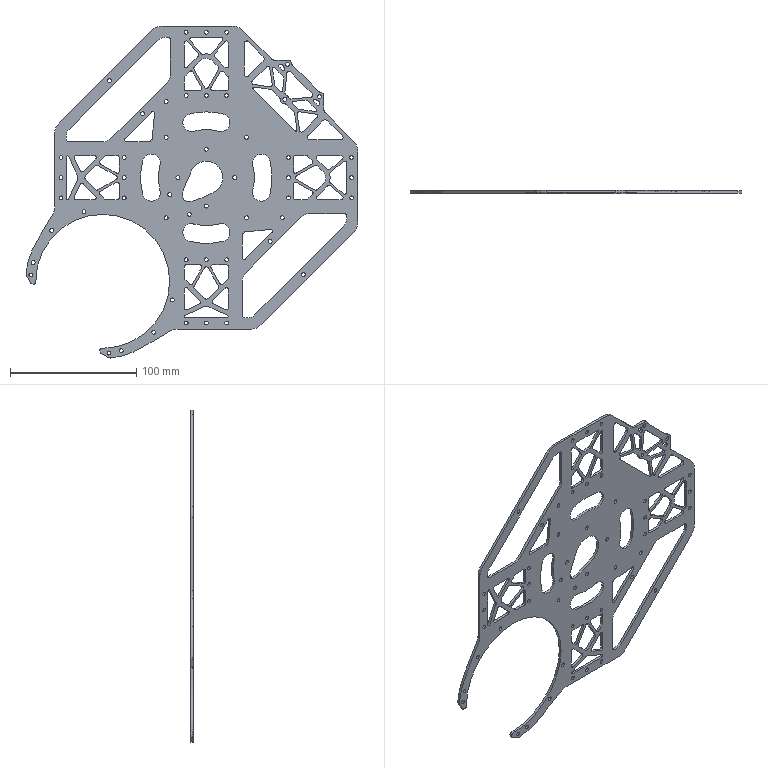Part | SolidWorks | features Fillet 6, ICE 2, Extrusion 1 | 1 solid | 484 faces | box 262.722 x 2 x 262.722 mm | volume 50644 mm3 | cylinder 320 | plane 155 | spline 9 | commonest cylinder face diameters 3.2 x123 3.1 x54 3 x48 6 x20 2 x16 14 x12